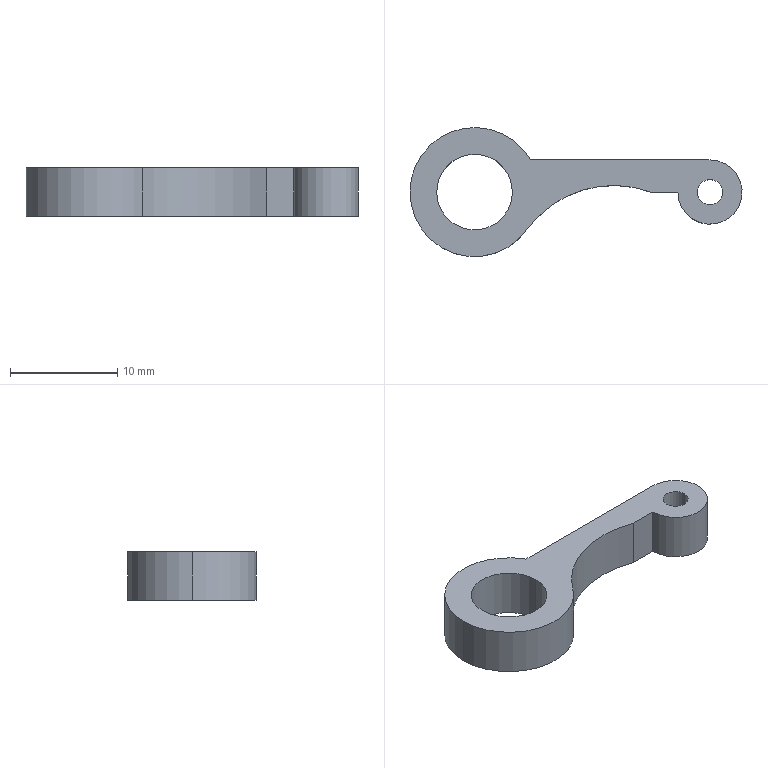Part | SolidWorks | features Extrusion 1 | 1 solid | 12 faces | box 31.031 x 12.062 x 4.5 mm | volume 635.986 mm3 | cylinder 8 | plane 4 | commonest cylinder face diameters 2.352 x2 7.08 x2 12.062 x2 6 x1 20 x1
STEP:
#1=CARTESIAN_POINT('',(20.824,0.,4.5));
#2=VERTEX_POINT('',#1);
#3=CARTESIAN_POINT('',(23.176,0.,4.5));
#4=VERTEX_POINT('',#3);
#5=CARTESIAN_POINT('',(22.,0.,4.5));
#6=DIRECTION('',(0.,0.,1.));
#7=DIRECTION('',(1.,0.,0.));
#8=AXIS2_PLACEMENT_3D('',#5,#6,#7);
#9=CIRCLE('',#8,1.176);
#10=EDGE_CURVE('',#2,#4,#9,.T.);
#11=ORIENTED_EDGE('',*,*,#10,.T.);
#12=CARTESIAN_POINT('',(23.176,0.,0.));
#13=VERTEX_POINT('',#12);
#14=CARTESIAN_POINT('',(23.176,0.,4.5));
#15=DIRECTION('',(0.,0.,-1.));
#16=VECTOR('',#15,1000.);
#17=LINE('',#14,#16);
#18=EDGE_CURVE('',#4,#13,#17,.T.);
#19=ORIENTED_EDGE('',*,*,#18,.T.);
#20=CARTESIAN_POINT('',(20.824,0.,0.));
#21=VERTEX_POINT('',#20);
#22=CARTESIAN_POINT('',(22.,0.,0.));
#23=DIRECTION('',(0.,0.,1.));
#24=DIRECTION('',(1.,0.,0.));
#25=AXIS2_PLACEMENT_3D('',#22,#23,#24);
#26=CIRCLE('',#25,1.176);
#27=EDGE_CURVE('',#21,#13,#26,.T.);
#28=ORIENTED_EDGE('',*,*,#27,.F.);
#29=CARTESIAN_POINT('',(20.824,0.,4.5));
#30=DIRECTION('',(0.,0.,-1.));
#31=VECTOR('',#30,1000.);
#32=LINE('',#29,#31);
#33=EDGE_CURVE('',#2,#21,#32,.T.);
#34=ORIENTED_EDGE('',*,*,#33,.F.);
#35=EDGE_LOOP('',(#11,#19,#28,#34));
#36=FACE_OUTER_BOUND('',#35,.T.);
#37=CARTESIAN_POINT('',(22.,0.,4.5));
#38=DIRECTION('',(0.,0.,-1.));
#39=DIRECTION('',(-1.,0.,0.));
#40=AXIS2_PLACEMENT_3D('',#37,#38,#39);
#41=CYLINDRICAL_SURFACE('',#40,1.176);
#42=ADVANCED_FACE('',(#36),#41,.F.);
#43=CARTESIAN_POINT('',(-3.54,0.,4.5));
#44=VERTEX_POINT('',#43);
#45=CARTESIAN_POINT('',(3.54,0.,4.5));
#46=VERTEX_POINT('',#45);
#47=CARTESIAN_POINT('',(0.,0.,4.5));
#48=DIRECTION('',(0.,0.,1.));
#49=DIRECTION('',(1.,0.,0.));
#50=AXIS2_PLACEMENT_3D('',#47,#48,#49);
#51=CIRCLE('',#50,3.54);
#52=EDGE_CURVE('',#44,#46,#51,.T.);
#53=ORIENTED_EDGE('',*,*,#52,.T.);
#54=CARTESIAN_POINT('',(3.54,0.,0.));
#55=VERTEX_POINT('',#54);
#56=CARTESIAN_POINT('',(3.54,0.,4.5));
#57=DIRECTION('',(0.,0.,-1.));
#58=VECTOR('',#57,1000.);
#59=LINE('',#56,#58);
#60=EDGE_CURVE('',#46,#55,#59,.T.);
#61=ORIENTED_EDGE('',*,*,#60,.T.);
#62=CARTESIAN_POINT('',(-3.54,0.,0.));
#63=VERTEX_POINT('',#62);
#64=CARTESIAN_POINT('',(0.,0.,0.));
#65=DIRECTION('',(0.,0.,1.));
#66=DIRECTION('',(1.,0.,0.));
#67=AXIS2_PLACEMENT_3D('',#64,#65,#66);
#68=CIRCLE('',#67,3.54);
#69=EDGE_CURVE('',#63,#55,#68,.T.);
#70=ORIENTED_EDGE('',*,*,#69,.F.);
#71=CARTESIAN_POINT('',(-3.54,0.,4.5));
#72=DIRECTION('',(0.,0.,-1.));
#73=VECTOR('',#72,1000.);
#74=LINE('',#71,#73);
#75=EDGE_CURVE('',#44,#63,#74,.T.);
#76=ORIENTED_EDGE('',*,*,#75,.F.);
#77=EDGE_LOOP('',(#53,#61,#70,#76));
#78=FACE_OUTER_BOUND('',#77,.T.);
#79=CARTESIAN_POINT('',(0.,0.,4.5));
#80=DIRECTION('',(0.,0.,-1.));
#81=DIRECTION('',(-1.,0.,0.));
#82=AXIS2_PLACEMENT_3D('',#79,#80,#81);
#83=CYLINDRICAL_SURFACE('',#82,3.54);
#84=ADVANCED_FACE('',(#78),#83,.F.);
#85=CARTESIAN_POINT('',(-6.031,0.,4.5));
#86=VERTEX_POINT('',#85);
#87=CARTESIAN_POINT('',(4.891,-3.529,4.5));
#88=VERTEX_POINT('',#87);
#89=CARTESIAN_POINT('',(0.,0.,4.5));
#90=DIRECTION('',(0.,0.,1.));
#91=DIRECTION('',(1.,0.,0.));
#92=AXIS2_PLACEMENT_3D('',#89,#90,#91);
#93=CIRCLE('',#92,6.031);
#94=EDGE_CURVE('',#86,#88,#93,.T.);
#95=ORIENTED_EDGE('',*,*,#94,.F.);
#96=CARTESIAN_POINT('',(-6.031,0.,0.));
#97=VERTEX_POINT('',#96);
#98=CARTESIAN_POINT('',(-6.031,0.,4.5));
#99=DIRECTION('',(0.,0.,-1.));
#100=VECTOR('',#99,1000.);
#101=LINE('',#98,#100);
#102=EDGE_CURVE('',#86,#97,#101,.T.);
#103=ORIENTED_EDGE('',*,*,#102,.T.);
#104=CARTESIAN_POINT('',(4.891,-3.529,0.));
#105=VERTEX_POINT('',#104);
#106=CARTESIAN_POINT('',(0.,0.,0.));
#107=DIRECTION('',(0.,0.,1.));
#108=DIRECTION('',(1.,0.,0.));
#109=AXIS2_PLACEMENT_3D('',#106,#107,#108);
#110=CIRCLE('',#109,6.031);
#111=EDGE_CURVE('',#97,#105,#110,.T.);
#112=ORIENTED_EDGE('',*,*,#111,.T.);
#113=CARTESIAN_POINT('',(4.891,-3.529,4.5));
#114=DIRECTION('',(0.,0.,-1.));
#115=VECTOR('',#114,1000.);
#116=LINE('',#113,#115);
#117=EDGE_CURVE('',#88,#105,#116,.T.);
#118=ORIENTED_EDGE('',*,*,#117,.F.);
#119=EDGE_LOOP('',(#95,#103,#112,#118));
#120=FACE_OUTER_BOUND('',#119,.T.);
#121=CARTESIAN_POINT('',(0.,0.,4.5));
#122=DIRECTION('',(0.,0.,-1.));
#123=DIRECTION('',(-1.,0.,0.));
#124=AXIS2_PLACEMENT_3D('',#121,#122,#123);
#125=CYLINDRICAL_SURFACE('',#124,6.031);
#126=ADVANCED_FACE('',(#120),#125,.T.);
#127=ORIENTED_EDGE('',*,*,#102,.F.);
#128=CARTESIAN_POINT('',(5.232,3.,4.5));
#129=VERTEX_POINT('',#128);
#130=CARTESIAN_POINT('',(0.,0.,4.5));
#131=DIRECTION('',(0.,0.,1.));
#132=DIRECTION('',(1.,0.,0.));
#133=AXIS2_PLACEMENT_3D('',#130,#131,#132);
#134=CIRCLE('',#133,6.031);
#135=EDGE_CURVE('',#129,#86,#134,.T.);
#136=ORIENTED_EDGE('',*,*,#135,.F.);
#137=CARTESIAN_POINT('',(5.232,3.,0.));
#138=VERTEX_POINT('',#137);
#139=CARTESIAN_POINT('',(5.232,3.,4.5));
#140=DIRECTION('',(0.,0.,-1.));
#141=VECTOR('',#140,1000.);
#142=LINE('',#139,#141);
#143=EDGE_CURVE('',#129,#138,#142,.T.);
#144=ORIENTED_EDGE('',*,*,#143,.T.);
#145=CARTESIAN_POINT('',(0.,0.,0.));
#146=DIRECTION('',(0.,0.,1.));
#147=DIRECTION('',(1.,0.,0.));
#148=AXIS2_PLACEMENT_3D('',#145,#146,#147);
#149=CIRCLE('',#148,6.031);
#150=EDGE_CURVE('',#138,#97,#149,.T.);
#151=ORIENTED_EDGE('',*,*,#150,.T.);
#152=EDGE_LOOP('',(#127,#136,#144,#151));
#153=FACE_OUTER_BOUND('',#152,.T.);
#154=CARTESIAN_POINT('',(0.,0.,4.5));
#155=DIRECTION('',(0.,0.,-1.));
#156=DIRECTION('',(-1.,0.,0.));
#157=AXIS2_PLACEMENT_3D('',#154,#155,#156);
#158=CYLINDRICAL_SURFACE('',#157,6.031);
#159=ADVANCED_FACE('',(#153),#158,.T.);
#160=CARTESIAN_POINT('',(16.464,0.,0.));
#161=VERTEX_POINT('',#160);
#162=CARTESIAN_POINT('',(13.,-9.381,0.));
#163=DIRECTION('',(0.,0.,1.));
#164=DIRECTION('',(1.,0.,0.));
#165=AXIS2_PLACEMENT_3D('',#162,#163,#164);
#166=CIRCLE('',#165,10.);
#167=EDGE_CURVE('',#161,#105,#166,.T.);
#168=ORIENTED_EDGE('',*,*,#167,.F.);
#169=CARTESIAN_POINT('',(16.464,0.,4.5));
#170=VERTEX_POINT('',#169);
#171=CARTESIAN_POINT('',(16.464,0.,4.5));
#172=DIRECTION('',(0.,0.,-1.));
#173=VECTOR('',#172,1000.);
#174=LINE('',#171,#173);
#175=EDGE_CURVE('',#170,#161,#174,.T.);
#176=ORIENTED_EDGE('',*,*,#175,.F.);
#177=CARTESIAN_POINT('',(13.,-9.381,4.5));
#178=DIRECTION('',(0.,0.,1.));
#179=DIRECTION('',(1.,0.,0.));
#180=AXIS2_PLACEMENT_3D('',#177,#178,#179);
#181=CIRCLE('',#180,10.);
#182=EDGE_CURVE('',#170,#88,#181,.T.);
#183=ORIENTED_EDGE('',*,*,#182,.T.);
#184=ORIENTED_EDGE('',*,*,#117,.T.);
#185=EDGE_LOOP('',(#168,#176,#183,#184));
#186=FACE_OUTER_BOUND('',#185,.T.);
#187=CARTESIAN_POINT('',(13.,-9.381,4.5));
#188=DIRECTION('',(0.,0.,-1.));
#189=DIRECTION('',(-1.,0.,0.));
#190=AXIS2_PLACEMENT_3D('',#187,#188,#189);
#191=CYLINDRICAL_SURFACE('',#190,10.);
#192=ADVANCED_FACE('',(#186),#191,.F.);
#193=CARTESIAN_POINT('',(19.,0.,0.));
#194=VERTEX_POINT('',#193);
#195=CARTESIAN_POINT('',(0.,0.,0.));
#196=DIRECTION('',(1.,0.,0.));
#197=VECTOR('',#196,1000.);
#198=LINE('',#195,#197);
#199=EDGE_CURVE('',#161,#194,#198,.T.);
#200=ORIENTED_EDGE('',*,*,#199,.T.);
#201=CARTESIAN_POINT('',(19.,0.,4.5));
#202=VERTEX_POINT('',#201);
#203=CARTESIAN_POINT('',(19.,0.,4.5));
#204=DIRECTION('',(0.,0.,-1.));
#205=VECTOR('',#204,1000.);
#206=LINE('',#203,#205);
#207=EDGE_CURVE('',#202,#194,#206,.T.);
#208=ORIENTED_EDGE('',*,*,#207,.F.);
#209=CARTESIAN_POINT('',(0.,0.,4.5));
#210=DIRECTION('',(1.,0.,0.));
#211=VECTOR('',#210,1000.);
#212=LINE('',#209,#211);
#213=EDGE_CURVE('',#170,#202,#212,.T.);
#214=ORIENTED_EDGE('',*,*,#213,.F.);
#215=ORIENTED_EDGE('',*,*,#175,.T.);
#216=EDGE_LOOP('',(#200,#208,#214,#215));
#217=FACE_OUTER_BOUND('',#216,.T.);
#218=CARTESIAN_POINT('',(0.,0.,4.5));
#219=DIRECTION('',(0.,1.,0.));
#220=DIRECTION('',(0.,0.,1.));
#221=AXIS2_PLACEMENT_3D('',#218,#219,#220);
#222=PLANE('',#221);
#223=ADVANCED_FACE('',(#217),#222,.F.);
#224=CARTESIAN_POINT('',(22.,3.,0.));
#225=VERTEX_POINT('',#224);
#226=CARTESIAN_POINT('',(22.,0.,0.));
#227=DIRECTION('',(0.,0.,1.));
#228=DIRECTION('',(1.,0.,0.));
#229=AXIS2_PLACEMENT_3D('',#226,#227,#228);
#230=CIRCLE('',#229,3.);
#231=EDGE_CURVE('',#194,#225,#230,.T.);
#232=ORIENTED_EDGE('',*,*,#231,.T.);
#233=CARTESIAN_POINT('',(22.,3.,4.5));
#234=VERTEX_POINT('',#233);
#235=CARTESIAN_POINT('',(22.,3.,4.5));
#236=DIRECTION('',(0.,0.,-1.));
#237=VECTOR('',#236,1000.);
#238=LINE('',#235,#237);
#239=EDGE_CURVE('',#234,#225,#238,.T.);
#240=ORIENTED_EDGE('',*,*,#239,.F.);
#241=CARTESIAN_POINT('',(22.,0.,4.5));
#242=DIRECTION('',(0.,0.,1.));
#243=DIRECTION('',(1.,0.,0.));
#244=AXIS2_PLACEMENT_3D('',#241,#242,#243);
#245=CIRCLE('',#244,3.);
#246=EDGE_CURVE('',#202,#234,#245,.T.);
#247=ORIENTED_EDGE('',*,*,#246,.F.);
#248=ORIENTED_EDGE('',*,*,#207,.T.);
#249=EDGE_LOOP('',(#232,#240,#247,#248));
#250=FACE_OUTER_BOUND('',#249,.T.);
#251=CARTESIAN_POINT('',(22.,0.,4.5));
#252=DIRECTION('',(0.,0.,-1.));
#253=DIRECTION('',(-1.,0.,0.));
#254=AXIS2_PLACEMENT_3D('',#251,#252,#253);
#255=CYLINDRICAL_SURFACE('',#254,3.);
#256=ADVANCED_FACE('',(#250),#255,.T.);
#257=ORIENTED_EDGE('',*,*,#60,.F.);
#258=CARTESIAN_POINT('',(0.,0.,4.5));
#259=DIRECTION('',(0.,0.,1.));
#260=DIRECTION('',(1.,0.,0.));
#261=AXIS2_PLACEMENT_3D('',#258,#259,#260);
#262=CIRCLE('',#261,3.54);
#263=EDGE_CURVE('',#46,#44,#262,.T.);
#264=ORIENTED_EDGE('',*,*,#263,.T.);
#265=ORIENTED_EDGE('',*,*,#75,.T.);
#266=CARTESIAN_POINT('',(0.,0.,0.));
#267=DIRECTION('',(0.,0.,1.));
#268=DIRECTION('',(1.,0.,0.));
#269=AXIS2_PLACEMENT_3D('',#266,#267,#268);
#270=CIRCLE('',#269,3.54);
#271=EDGE_CURVE('',#55,#63,#270,.T.);
#272=ORIENTED_EDGE('',*,*,#271,.F.);
#273=EDGE_LOOP('',(#257,#264,#265,#272));
#274=FACE_OUTER_BOUND('',#273,.T.);
#275=CARTESIAN_POINT('',(0.,0.,4.5));
#276=DIRECTION('',(0.,0.,-1.));
#277=DIRECTION('',(-1.,0.,0.));
#278=AXIS2_PLACEMENT_3D('',#275,#276,#277);
#279=CYLINDRICAL_SURFACE('',#278,3.54);
#280=ADVANCED_FACE('',(#274),#279,.F.);
#281=CARTESIAN_POINT('',(0.,3.,0.));
#282=DIRECTION('',(-1.,0.,0.));
#283=VECTOR('',#282,1000.);
#284=LINE('',#281,#283);
#285=EDGE_CURVE('',#225,#138,#284,.T.);
#286=ORIENTED_EDGE('',*,*,#285,.T.);
#287=ORIENTED_EDGE('',*,*,#143,.F.);
#288=CARTESIAN_POINT('',(0.,3.,4.5));
#289=DIRECTION('',(-1.,0.,0.));
#290=VECTOR('',#289,1000.);
#291=LINE('',#288,#290);
#292=EDGE_CURVE('',#234,#129,#291,.T.);
#293=ORIENTED_EDGE('',*,*,#292,.F.);
#294=ORIENTED_EDGE('',*,*,#239,.T.);
#295=EDGE_LOOP('',(#286,#287,#293,#294));
#296=FACE_OUTER_BOUND('',#295,.T.);
#297=CARTESIAN_POINT('',(0.,3.,4.5));
#298=DIRECTION('',(0.,-1.,0.));
#299=DIRECTION('',(1.,0.,0.));
#300=AXIS2_PLACEMENT_3D('',#297,#298,#299);
#301=PLANE('',#300);
#302=ADVANCED_FACE('',(#296),#301,.F.);
#303=ORIENTED_EDGE('',*,*,#18,.F.);
#304=CARTESIAN_POINT('',(22.,0.,4.5));
#305=DIRECTION('',(0.,0.,1.));
#306=DIRECTION('',(1.,0.,0.));
#307=AXIS2_PLACEMENT_3D('',#304,#305,#306);
#308=CIRCLE('',#307,1.176);
#309=EDGE_CURVE('',#4,#2,#308,.T.);
#310=ORIENTED_EDGE('',*,*,#309,.T.);
#311=ORIENTED_EDGE('',*,*,#33,.T.);
#312=CARTESIAN_POINT('',(22.,0.,0.));
#313=DIRECTION('',(0.,0.,1.));
#314=DIRECTION('',(1.,0.,0.));
#315=AXIS2_PLACEMENT_3D('',#312,#313,#314);
#316=CIRCLE('',#315,1.176);
#317=EDGE_CURVE('',#13,#21,#316,.T.);
#318=ORIENTED_EDGE('',*,*,#317,.F.);
#319=EDGE_LOOP('',(#303,#310,#311,#318));
#320=FACE_OUTER_BOUND('',#319,.T.);
#321=CARTESIAN_POINT('',(22.,0.,4.5));
#322=DIRECTION('',(0.,0.,-1.));
#323=DIRECTION('',(-1.,0.,0.));
#324=AXIS2_PLACEMENT_3D('',#321,#322,#323);
#325=CYLINDRICAL_SURFACE('',#324,1.176);
#326=ADVANCED_FACE('',(#320),#325,.F.);
#327=ORIENTED_EDGE('',*,*,#135,.T.);
#328=ORIENTED_EDGE('',*,*,#94,.T.);
#329=ORIENTED_EDGE('',*,*,#182,.F.);
#330=ORIENTED_EDGE('',*,*,#213,.T.);
#331=ORIENTED_EDGE('',*,*,#246,.T.);
#332=ORIENTED_EDGE('',*,*,#292,.T.);
#333=EDGE_LOOP('',(#327,#328,#329,#330,#331,#332));
#334=FACE_OUTER_BOUND('',#333,.T.);
#335=ORIENTED_EDGE('',*,*,#52,.F.);
#336=ORIENTED_EDGE('',*,*,#263,.F.);
#337=EDGE_LOOP('',(#335,#336));
#338=FACE_BOUND('',#337,.T.);
#339=ORIENTED_EDGE('',*,*,#10,.F.);
#340=ORIENTED_EDGE('',*,*,#309,.F.);
#341=EDGE_LOOP('',(#339,#340));
#342=FACE_BOUND('',#341,.T.);
#343=CARTESIAN_POINT('',(0.,0.,4.5));
#344=DIRECTION('',(0.,0.,1.));
#345=DIRECTION('',(1.,0.,0.));
#346=AXIS2_PLACEMENT_3D('',#343,#344,#345);
#347=PLANE('',#346);
#348=ADVANCED_FACE('',(#334,#338,#342),#347,.T.);
#349=ORIENTED_EDGE('',*,*,#150,.F.);
#350=ORIENTED_EDGE('',*,*,#285,.F.);
#351=ORIENTED_EDGE('',*,*,#231,.F.);
#352=ORIENTED_EDGE('',*,*,#199,.F.);
#353=ORIENTED_EDGE('',*,*,#167,.T.);
#354=ORIENTED_EDGE('',*,*,#111,.F.);
#355=EDGE_LOOP('',(#349,#350,#351,#352,#353,#354));
#356=FACE_OUTER_BOUND('',#355,.T.);
#357=ORIENTED_EDGE('',*,*,#69,.T.);
#358=ORIENTED_EDGE('',*,*,#271,.T.);
#359=EDGE_LOOP('',(#357,#358));
#360=FACE_BOUND('',#359,.T.);
#361=ORIENTED_EDGE('',*,*,#27,.T.);
#362=ORIENTED_EDGE('',*,*,#317,.T.);
#363=EDGE_LOOP('',(#361,#362));
#364=FACE_BOUND('',#363,.T.);
#365=CARTESIAN_POINT('',(0.,0.,0.));
#366=DIRECTION('',(0.,0.,1.));
#367=DIRECTION('',(1.,0.,0.));
#368=AXIS2_PLACEMENT_3D('',#365,#366,#367);
#369=PLANE('',#368);
#370=ADVANCED_FACE('',(#356,#360,#364),#369,.F.);
#371=CLOSED_SHELL('',(#42,#84,#126,#159,#192,#223,#256,#280,#302,#326,#348,#370));
#372=MANIFOLD_SOLID_BREP('',#371);
#373=CARTESIAN_POINT('',(0.,0.,0.));
#374=DIRECTION('',(0.,0.,1.));
#375=DIRECTION('',(1.,0.,0.));
#376=AXIS2_PLACEMENT_3D('',#373,#374,#375);
#377=(LENGTH_UNIT()NAMED_UNIT(*)SI_UNIT(.MILLI.,.METRE.));
#378=UNCERTAINTY_MEASURE_WITH_UNIT(LENGTH_MEASURE(0.00001),#377,'','');
#379=(NAMED_UNIT(*)PLANE_ANGLE_UNIT()SI_UNIT($,.RADIAN.));
#380=(NAMED_UNIT(*)SI_UNIT($,.STERADIAN.)SOLID_ANGLE_UNIT());
#381=(GEOMETRIC_REPRESENTATION_CONTEXT(3)GLOBAL_UNCERTAINTY_ASSIGNED_CONTEXT((#378))GLOBAL_UNIT_ASSIGNED_CONTEXT((#377,#379,#380))REPRESENTATION_CONTEXT('',''));
#382=ADVANCED_BREP_SHAPE_REPRESENTATION('',(#372,#376),#381);